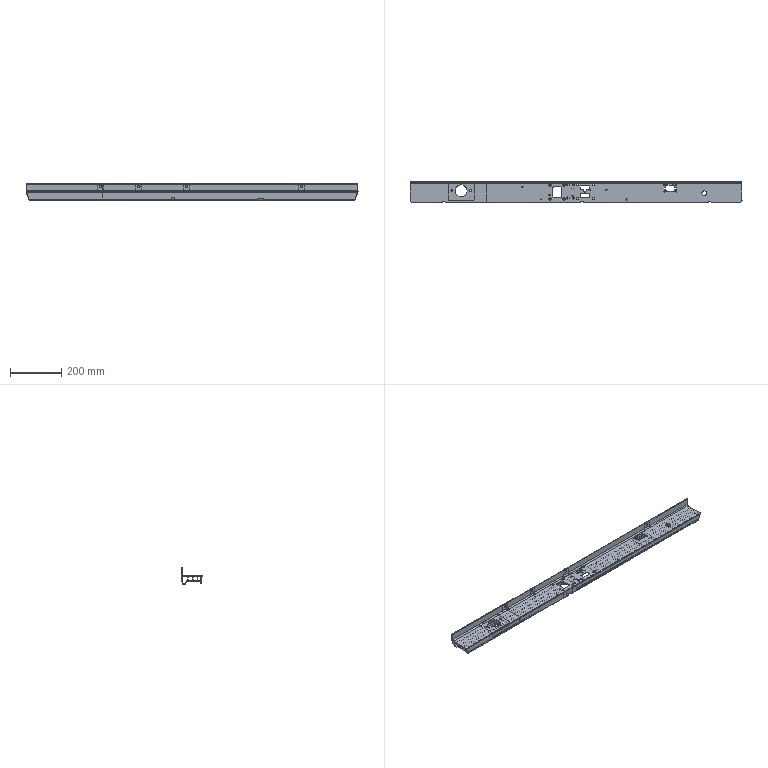NC program | NX | posted with a generic post | part box 1301 x 81.1 x 63 mm
Lines 13798 to 14822 of 19815:
(FIXED_CONTOUR_COPY , TOOL : D6)
N27582 T06 M6
N27584 G54
N27586 G17 G0 G90 X222.672 Y-32.604 B0. C0. S9500 M3
N27588 G43 Z30. H6
N27590 Z3.6
N27592 G94 G1 Z-0.54 F1000.
N27594 G2 X222.372 Y-32.084 R0.6
N27596 G1 Y-31.745 Z-0.522 F2500.
N27598 Y-31.55 Z-0.514
N27600 Y-31.069 Z-0.503
N27602 Y-30.589 Z-0.501
N27604 Y-30.108 Z-0.509
N27606 Y-29.559 Z-0.53
N27608 X222.401 Y-29.379 Z-0.579
N27610 X222.462 Y-29.117 Z-0.676
N27612 X222.481 Y-29.051 Z-0.705
N27614 Y-29.628 Z-0.675
N27616 Y-30.108 Z-0.657
N27618 Y-30.589 Z-0.647
N27620 Y-31.069 Z-0.648
N27622 Y-31.55 Z-0.659
N27624 Y-32.03 Z-0.681
N27626 Y-32.555 Z-0.715
N27628 X222.538 Y-32.748 Z-0.807
N27630 X222.61 Y-32.979 Z-0.916
N27632 X222.62 Y-33.005 Z-0.929
N27634 Y-32.489 Z-0.893
N27636 Y-32.03 Z-0.864
N27638 Y-31.739 Z-0.85
N27640 Y-31.55 Z-0.843
N27642 Y-31.069 Z-0.832
N27644 Y-30.589 Z-0.833
N27646 Y-30.108 Z-0.843
N27648 Y-29.65 Z-0.862
N27650 Y-28.617 Z-0.918
N27652 X222.719 Y-28.379 Z-1.062
N27654 X222.778 Y-28.245 Z-1.143
N27656 Y-28.438 Z-1.137
N27658 Y-28.909 Z-1.116
N27660 Y-29.628 Z-1.075
N27662 Y-30.108 Z-1.054
N27664 Y-30.589 Z-1.042
N27666 Y-31.069
N27668 Y-31.675 Z-1.058
N27670 Y-32.03 Z-1.075
N27672 Y-32.334 Z-1.094
N27674 Y-32.511 Z-1.103
N27676 Y-32.815 Z-1.125
N27678 Y-32.992 Z-1.132
N27680 Y-33.381 Z-1.153
N27682 X222.818 Y-33.463 Z-1.209
N27684 X222.95 Y-33.7 Z-1.384
N27686 Y-33.24 Z-1.368
N27688 Y-32.992 Z-1.355
N27690 Y-32.646 Z-1.341
N27692 Y-32.511 Z-1.331
N27694 Y-32.165 Z-1.314
N27696 Y-32.03 Z-1.305
N27698 Y-31.55 Z-1.283
N27700 Y-31.069 Z-1.271
N27702 Y-30.589 Z-1.272
N27704 Y-30.108 Z-1.284
N27706 Y-29.493 Z-1.314
N27708 Y-29.013 Z-1.341
N27710 Y-28.566 Z-1.361
N27712 Y-28.139 Z-1.369
N27714 Y-27.914 Z-1.372
N27716 X223.09 Y-27.662 Z-1.556
N27718 X223.127 Y-27.6 Z-1.603
N27720 Y-28.403 Z-1.594
N27722 Y-28.706 Z-1.589
N27724 Y-29.186 Z-1.569
N27726 Y-29.628 Z-1.543
N27728 Y-30.108 Z-1.52
N27730 Y-30.589 Z-1.506
N27732 Y-31.069
N27734 Y-31.55 Z-1.519
N27736 Y-32.511 Z-1.564
N27738 Y-32.992 Z-1.582
N27740 Y-33.472 Z-1.596
N27742 Y-33.953 Z-1.614
N27744 Y-34.011 Z-1.615
N27746 X223.153 Y-34.055 Z-1.649
N27748 X223.307 Y-34.181 Z-1.838
N27750 Y-33.738 Z-1.833
N27752 Y-33.207 Z-1.814
N27754 Y-32.776 Z-1.807
N27756 Y-32.511 Z-1.797
N27758 Y-32.295 Z-1.792
N27760 Y-32.03 Z-1.779
N27762 Y-31.55 Z-1.759
N27764 Y-31.069 Z-1.746
N27766 Y-30.589
N27768 Y-30.108 Z-1.76
N27770 Y-29.628 Z-1.783
N27772 Y-29.363 Z-1.798
N27774 Y-29.147 Z-1.804
N27776 Y-28.883 Z-1.815
N27778 Y-28.402 Z-1.823
N27780 Y-27.922 Z-1.828
N27782 Y-27.453 Z-1.826
N27784 Y-27.422 Z-1.827
N27786 X223.487 Y-27.271 Z-2.05
N27788 Y-28.099 Z-2.054
N27790 Y-28.614 Z-2.049
N27792 Y-29.06 Z-2.042
N27794 Y-29.54 Z-2.027
N27796 Y-30.108 Z-1.999
N27798 Y-30.589 Z-1.985
N27800 Y-31.069
N27802 Y-31.55 Z-1.999
N27804 Y-32.118 Z-2.022
N27806 Y-32.511 Z-2.03
N27808 Y-32.599 Z-2.034
N27810 Y-32.992 Z-2.041
N27812 Y-33.384 Z-2.045
N27814 Y-33.56 Z-2.052
N27816 Y-33.953 Z-2.054
N27818 Y-34.329 Z-2.059
N27820 X223.667 Y-34.478 Z-2.281
N27822 Y-33.863 Z-2.274
N27824 Y-33.383 Z-2.272
N27826 Y-32.992 Z-2.268
N27828 Y-32.6 Z-2.26
N27830 Y-32.511
N27832 Y-32.03 Z-2.252
N27834 Y-31.941
N27836 Y-31.55 Z-2.237
N27838 Y-31.069 Z-2.225
N27840 Y-30.589
N27842 Y-30.108 Z-2.238
N27844 Y-29.717 Z-2.257
N27846 Y-29.539 Z-2.258
N27848 Y-29.147 Z-2.268
N27850 Y-29.058
N27852 Y-28.667 Z-2.275
N27854 Y-28.276 Z-2.278
N27856 Y-27.617 Z-2.276
N27858 Y-27.121 Z-2.272
N27860 X223.848 Y-26.971 Z-2.494
N27862 Y-27.439 Z-2.498
N27864 Y-28.453 Z-2.499
N27866 Y-28.881 Z-2.494
N27868 Y-29.147
N27870 Y-29.361 Z-2.489
N27872 Y-29.895 Z-2.486
N27874 Y-30.108 Z-2.476
N27876 Y-30.589 Z-2.464
N27878 Y-31.069
N27880 Y-31.283 Z-2.471
N27882 Y-31.55 Z-2.474
N27884 Y-31.764 Z-2.482
N27886 Y-32.297 Z-2.483
N27888 Y-32.511 Z-2.488
N27890 Y-32.778
N27892 Y-33.205 Z-2.494
N27894 Y-33.953 Z-2.495
N27896 Y-34.626 Z-2.501
N27898 X224.029 Y-34.774 Z-2.722
N27900 Y-33.953 Z-2.717
N27902 Y-32.474 Z-2.714
N27904 Y-32.03 Z-2.712
N27906 Y-31.587
N27908 Y-31.069 Z-2.704
N27910 Y-30.552 Z-2.705
N27912 Y-30.072 Z-2.716
N27914 Y-29.628 Z-2.719
N27916 Y-28.63 Z-2.721
N27918 Y-27.225 Z-2.718
N27920 Y-26.821 Z-2.716
N27922 X224.211 Y-26.67 Z-2.941
N27924 Y-26.745 Z-2.937
N27926 Y-27.049 Z-2.942
N27928 Y-29.628 Z-2.946
N27930 Y-29.823 Z-2.944
N27932 Y-30.108 Z-2.946
N27934 Y-30.394 Z-2.945
N27936 Y-30.589 Z-2.941
N27938 Y-31.069 Z-2.942
N27940 Y-31.265 Z-2.945
N27942 Y-32.03 Z-2.94
N27944 Y-33.953 Z-2.941
N27946 Y-34.923 Z-2.943
N27948 X224.353 Y-35.038 Z-3.113
N27950 X224.4 Y-35.041 Z-3.168
N27952 Y-34.993 Z-3.165
N27954 Y-34.609 Z-3.167
N27956 Y-32.03 Z-3.169
N27958 Y-31.069 Z-3.175
N27960 Y-30.589 Z-3.173
N27962 Y-30.108 Z-3.175
N27964 Y-28.667 Z-3.169
N27966 Y-27.049 Z-3.168
N27968 Y-26.745 Z-3.162
N27970 Y-26.669 Z-3.166
N27972 Y-26.542
N27974 X224.555 Z-3.347
N27976 X224.598 Y-26.541 Z-3.39
N27978 Y-26.58 Z-3.388
N27980 Y-29.231 Z-3.391
N27982 Y-30.108 Z-3.395
N27984 Y-31.55
N27986 Y-32.511 Z-3.389
N27988 Y-35.054 Z-3.39
N27990 X224.81 Y-35.066 Z-3.602
N27992 Y-34.92 Z-3.597
N27994 Y-32.511
N27996 Y-31.55 Z-3.604
N27998 Y-31.089 Z-3.597
N28000 Y-30.57
N28002 Y-30.108 Z-3.604
N28004 Y-28.648 Z-3.597
N28006 Y-26.736
N28008 Y-26.53 Z-3.602
N28010 X225.034 Y-26.519 Z-3.791
N28012 Y-27.706 Z-3.792
N28014 Y-28.667
N28016 Y-29.628 Z-3.797
N28018 Y-31.848 Z-3.798
N28020 Y-32.49 Z-3.792
N28022 Y-34.433 Z-3.79
N28024 Y-35.074 Z-3.786
N28026 X225.136 Y-35.077 Z-3.858
N28028 X225.272 Y-35.082 Z-3.944
N28030 Y-34.4 Z-3.95
N28032 Y-32.958 Z-3.953
N28034 Y-32.511 Z-3.959
N28036 Y-31.977 Z-3.973
N28038 Y-31.82 Z-3.977
N28040 Y-31.55 Z-3.979
N28042 Y-30.075
N28044 Y-29.628 Z-3.967
N28046 Y-29.181 Z-3.959
N28048 Y-27.225 Z-3.95
N28050 Y-26.745 Z-3.953
N28052 Y-26.513 Z-3.957
N28054 X225.408 Y-26.511 Z-4.04
N28056 X225.523 Y-26.51 Z-4.107
N28058 Y-26.745 Z-4.104
N28060 Y-27.225 Z-4.102
N28062 Y-28.667 Z-4.108
N28064 Y-29.169 Z-4.112
N28066 Y-29.649 Z-4.124
N28068 Y-30.108 Z-4.143
N28070 Y-31.55
N28072 Y-31.84 Z-4.136
N28074 Y-32.028 Z-4.123
N28076 Y-32.511 Z-4.109
N28078 Y-32.992 Z-4.104
N28080 Y-34.433 Z-4.102
N28082 Y-35.087 Z-4.097
N28084 X225.781 Y-35.091 Z-4.25
N28086 Y-34.914 Z-4.247
N28088 Y-34.433 Z-4.249
N28090 Y-32.511 Z-4.251
N28092 Y-32.03 Z-4.264
N28094 Y-31.55 Z-4.293
N28096 Y-30.108
N28098 Y-29.628 Z-4.265
N28100 Y-29.147 Z-4.253
N28102 Y-26.743 Z-4.249
N28104 Y-26.507 Z-4.253
N28106 X226.047 Y-26.506 Z-4.386
N28108 Y-29.147
N28110 Y-29.651 Z-4.398
N28112 Y-30.108 Z-4.429
N28114 Y-31.55
N28116 Y-32.03 Z-4.395
N28118 Y-32.511 Z-4.387
N28120 Y-35.093 Z-4.386
N28122 X226.268 Y-35.095 Z-4.484
N28124 X226.322 Z-4.505
N28126 Y-34.954 Z-4.503
N28128 Y-32.405 Z-4.505
N28130 Y-32.03 Z-4.511
N28132 Y-31.55 Z-4.544
N28134 Y-31.444 Z-4.546
N28136 Y-30.108
N28138 Y-29.921 Z-4.528
N28140 Y-29.734 Z-4.52
N28142 Y-29.628 Z-4.514
N28144 Y-29.147 Z-4.504
N28146 Y-26.638
N28148 Y-26.504 Z-4.505
N28150 X226.512 Y-26.503 Z-4.58
N28152 X226.603 Z-4.609
N28154 Y-29.147 Z-4.608
N28156 Y-29.628 Z-4.616
N28158 Y-29.717 Z-4.619
N28160 Y-29.806 Z-4.627
N28162 Y-30.108 Z-4.646
N28164 Y-30.589 Z-4.649
N28166 Y-31.069
N28168 Y-31.55 Z-4.64
N28170 Y-32.03 Z-4.613
N28172 Y-32.511 Z-4.608
N28174 Y-34.948 Z-4.607
N28176 Y-35.097 Z-4.609
N28178 X226.89 Y-35.098 Z-4.694
N28180 Y-32.511
N28182 Y-32.03 Z-4.699
N28184 Y-31.769 Z-4.709
N28186 Y-31.55 Z-4.721
N28188 Y-31.288 Z-4.731
N28190 Y-31.069 Z-4.735
N28192 Y-30.37 Z-4.734
N28194 Y-30.108 Z-4.727
N28196 Y-29.999 Z-4.717
N28198 Y-29.628 Z-4.702
N28200 Y-29.147 Z-4.695
N28202 Y-26.502 Z-4.694
N28204 X227.001 Z-4.727
N28206 X227.182 Y-26.501 Z-4.761
N28208 Y-27.048 Z-4.76
N28210 Y-27.706 Z-4.762
N28212 Y-29.147 Z-4.763
N28214 Y-29.628 Z-4.771
N28216 Y-29.805 Z-4.777
N28218 Y-30.108 Z-4.792
N28220 Y-30.589 Z-4.8
N28222 Y-31.069
N28224 Y-31.423 Z-4.791
N28226 Y-32.03 Z-4.768
N28228 Y-32.511 Z-4.764
N28230 Y-34.914 Z-4.761
N28232 Y-35.099 Z-4.765
N28234 X227.476 Z-4.821
N28236 Y-34.448 Z-4.817
N28238 Y-32.496 Z-4.823
N28240 Y-32.001 Z-4.828
N28242 Y-31.55 Z-4.843
N28244 Y-31.069 Z-4.852
N28246 Y-30.559
N28248 Y-30.094 Z-4.847
N28250 Y-29.628 Z-4.831
N28252 Y-29.147 Z-4.822
N28254 Y-28.667 Z-4.817
N28256 Y-27.225 Z-4.818
N28258 Y-26.501 Z-4.813
N28260 X227.772 Y-26.5 Z-4.857
N28262 Y-26.732 Z-4.86
N28264 Y-27.225 Z-4.863
N28266 Y-28.739
N28268 Y-29.7 Z-4.873
N28270 Y-30.108 Z-4.883
N28272 Y-31.141 Z-4.884
N28274 Y-31.622 Z-4.878
N28276 Y-32.03 Z-4.869
N28278 Y-32.583 Z-4.865
N28280 Y-34.505 Z-4.862
N28282 Y-35.072 Z-4.866
N28284 Y-35.099 Z-4.863
N28286 X227.846 Y-35.1 Z-4.874
N28288 X227.98 Z-4.888
N28290 X228.07 Z-4.891
N28292 Y-33.953 Z-4.889
N28294 Y-32.03 Z-4.89
N28296 Y-31.069 Z-4.897
N28298 Y-30.108
N28300 Y-29.54 Z-4.893
N28302 Y-28.667 Z-4.889
N28304 Y-26.677 Z-4.888
N28306 Y-26.5 Z-4.891
N28308 X228.268 Z-4.897
N28310 X228.37 Z-4.899
N28312 Y-26.843 Z-4.897
N28314 Y-29.628 Z-4.898
N28316 Y-29.824 Z-4.9
N28318 Y-31.354
N28320 Y-32.03 Z-4.898
N28322 Y-35.1
N28324 X228.47 Z-4.9
N28326 X228.67
N28328 Y-26.5
N28330 X228.97
N28332 Y-35.1
N28334 X229.27
N28336 Y-26.5
N28338 X229.57
N28340 Y-35.1
N28342 X229.87
N28344 Y-26.5
N28346 X230.17
N28348 Y-35.1
N28350 X230.47
N28352 Y-26.5
N28354 X230.77
N28356 Y-35.1
N28358 X231.07
N28360 Y-26.5
N28362 X231.37
N28364 Y-35.1
N28366 X231.67
N28368 Y-26.5
N28370 X231.97
N28372 Y-35.1
N28374 X232.27
N28376 Y-26.5
N28378 X232.57
N28380 Y-35.1
N28382 X232.87
N28384 Y-26.5
N28386 X233.17
N28388 Y-35.1
N28390 X233.47
N28392 Y-26.5
N28394 X233.77
N28396 Y-35.1
N28398 X234.07
N28400 Y-26.5
N28402 X234.37
N28404 Y-35.1
N28406 X234.67
N28408 Y-26.5
N28410 X234.97
N28412 Y-35.1
N28414 X235.27
N28416 Y-26.5
N28418 X235.57
N28420 Y-35.1
N28422 X235.87
N28424 Y-26.5
N28426 X236.17
N28428 Y-35.1
N28430 X236.47
N28432 Y-26.5
N28434 X236.77
N28436 Y-35.1
N28438 X237.07
N28440 Y-26.5
N28442 X237.37
N28444 Y-35.1
N28446 X237.67
N28448 Y-26.5
N28450 X237.97
N28452 Y-35.1
N28454 X238.27
N28456 Y-26.5
N28458 X238.57
N28460 Y-35.1
N28462 X238.87 Z-4.899
N28464 Y-34.678 Z-4.9
N28466 Y-34.433 Z-4.897
N28468 Y-32.03 Z-4.898
N28470 Y-31.786 Z-4.9
N28472 Y-30.353
N28474 Y-30.108 Z-4.898
N28476 Y-26.5 Z-4.897
N28478 X239.17 Z-4.89
N28480 Y-27.642 Z-4.888
N28482 Y-29.628 Z-4.89
N28484 Y-30.589 Z-4.897
N28486 Y-31.55
N28488 Y-32.094 Z-4.892
N28490 Y-32.992 Z-4.888
N28492 Y-34.433
N28494 Y-34.561 Z-4.89
N28496 Y-34.931 Z-4.889
N28498 Y-35.101 Z-4.891
N28500 X239.23 Z-4.885
N28502 X239.236 Y-34.914
N28504 X239.237 Y-34.9
N28506 X239.308 Y-34.895 Z-4.876
N28508 X239.33 Y-34.887 Z-4.874
N28510 X239.336 Y-34.877 Z-4.873
N28512 X239.372 Y-34.844 Z-4.869
N28514 Y-35.1
N28516 X239.468 Z-4.854
N28518 Y-34.433 Z-4.86
N28520 Y-32.992
N28522 Y-32.008 Z-4.869
N28524 Y-31.55 Z-4.881
N28526 Y-30.589 Z-4.883
N28528 Y-30.086 Z-4.878
N28530 Y-29.606 Z-4.867
N28532 Y-29.147 Z-4.863
N28534 Y-27.225 Z-4.859
N28536 Y-26.723 Z-4.861
N28538 Y-26.5 Z-4.859
N28540 X239.724 Y-26.501 Z-4.824
N28542 X239.764 Z-4.817
N28544 Y-26.745 Z-4.813
N28546 Y-27.186 Z-4.812
N28548 Y-28.706 Z-4.815
N28550 Y-29.628 Z-4.824
N28552 Y-30.108 Z-4.84
N28554 Y-30.589 Z-4.848
N28556 Y-31.109 Z-4.846
N28558 Y-31.55 Z-4.84
N28560 Y-32.03 Z-4.824
N28562 Y-32.511 Z-4.816
N28564 Y-32.992 Z-4.813
N28566 Y-34.433
N28568 Y-34.947 Z-4.809
N28570 Y-35.099
N28572 X240.059 Y-35.098 Z-4.756
N28574 Y-34.585
N28576 Y-34.433 Z-4.757
N28578 Y-32.511 Z-4.758
N28580 Y-32.03 Z-4.765
N28582 Y-31.55 Z-4.783
N28584 Y-31.398 Z-4.785
N28586 Y-31.069 Z-4.796
N28588 Y-30.589
N28590 Y-30.284 Z-4.79
N28592 Y-29.628 Z-4.764
N28594 Y-28.995 Z-4.758
N28596 Y-26.745 Z-4.757
N28598 Y-26.501 Z-4.759
N28600 X240.214 Y-26.502 Z-4.727
N28602 X240.35 Z-4.687
N28604 Y-29.147
N28606 Y-29.628 Z-4.693
N28608 Y-29.841 Z-4.702
N28610 Y-30.108 Z-4.718
N28612 Y-30.322 Z-4.725
N28614 Y-30.589 Z-4.728
N28616 Y-31.069
N28618 Y-31.337 Z-4.724
N28620 Y-31.55 Z-4.716
N28622 Y-31.817 Z-4.701
N28624 Y-32.03 Z-4.693
N28626 Y-32.645 Z-4.688
N28628 Y-35.028 Z-4.687
N28630 Y-35.098 Z-4.688
N28632 X240.637 Y-35.096 Z-4.6
N28634 Y-32.446 Z-4.601
N28636 Y-32.03 Z-4.606
N28638 Y-31.55 Z-4.634
N28640 Y-31.069 Z-4.642
N28642 Y-30.459 Z-4.641
N28644 Y-30.108 Z-4.637
N28646 Y-29.628 Z-4.608
N28648 Y-29.147 Z-4.601
N28650 Y-26.503
N28652 X240.703 Z-4.58
N28654 X240.916 Y-26.504 Z-4.496
N28656 Y-26.714 Z-4.494
N28658 Y-29.209 Z-4.495
N28660 Y-29.628 Z-4.505
N28662 Y-29.899 Z-4.517
N28664 Y-30.108 Z-4.537
N28666 Y-31.069
N28668 Y-31.55 Z-4.535
N28670 Y-31.76 Z-4.513
N28672 Y-32.03 Z-4.502
N28674 Y-32.511 Z-4.494
N28676 Y-34.937
N28678 Y-35.095 Z-4.496
N28680 X241.039 Y-35.094 Z-4.444
N28682 X241.191 Y-35.093 Z-4.375
N28684 Y-32.511 Z-4.376
N28686 Y-32.029 Z-4.384
N28688 Y-31.55 Z-4.418
N28690 Y-30.108 Z-4.42
N28692 Y-29.628 Z-4.388
N28694 Y-29.145 Z-4.378
N28696 Y-26.505 Z-4.376
N28698 X241.456 Y-26.507 Z-4.238
N28700 Y-26.782 Z-4.236
N28702 Y-27.225 Z-4.238
N28704 Y-28.704
N28706 Y-29.147 Z-4.241
N28708 Y-29.628 Z-4.257
N28710 Y-30.108 Z-4.281
N28712 Y-31.55
N28714 Y-32.03 Z-4.25
N28716 Y-32.511 Z-4.241
N28718 Y-32.992 Z-4.239
N28720 Y-33.915
N28722 Y-34.914 Z-4.236
N28724 Y-35.09 Z-4.24
N28726 X241.683 Y-35.088 Z-4.11
N28728 X241.714 Y-35.087 Z-4.092
N28730 Y-34.433 Z-4.087
N28732 Y-32.511 Z-4.097
N28734 Y-31.966 Z-4.109
N28736 Y-31.55 Z-4.129
N28738 Y-30.108
N28740 Y-29.781 Z-4.123
N28742 Y-29.628 Z-4.114
N28744 Y-29.147 Z-4.098
N28746 Y-28.667 Z-4.092
N28748 Y-27.225 Z-4.091
N28750 Y-26.509 Z-4.085
N28752 X241.964 Y-26.513 Z-3.937
N28754 Y-26.553
N28756 Y-26.561 Z-3.935
N28758 Y-27.225 Z-3.94
N28760 Y-28.741 Z-3.941
N28762 Y-29.147 Z-3.946
N28764 Y-29.554 Z-3.958
N28766 Y-29.832 Z-3.962
N28768 Y-31.624
N28770 Y-32.03 Z-3.95
N28772 Y-32.511 Z-3.942
N28774 Y-34.433 Z-3.932
N28776 Y-34.914 Z-3.935
N28778 Y-35.083 Z-3.939
N28780 X242.138 Y-35.078 Z-3.818
N28782 X242.201 Y-35.074 Z-3.769
N28784 Y-34.374 Z-3.766
N28786 Y-32.511 Z-3.775
N28788 Y-31.55 Z-3.78
N28790 Y-30.529
N28792 Y-29.762
N28794 Y-29.147 Z-3.774
N28796 Y-27.706 Z-3.773
N28798 Y-26.523 Z-3.774
N28800 X242.425 Y-26.537 Z-3.584
N28802 Y-26.736 Z-3.579
N28804 Y-29.147 Z-3.58
N28806 Y-30.108 Z-3.586
N28808 Y-30.571 Z-3.579
N28810 Y-31.087
N28812 Y-31.55 Z-3.586
N28814 Y-32.511 Z-3.58
N28816 Y-34.931
N28818 Y-35.058 Z-3.584
N28820 X242.486 Y-35.052 Z-3.525
N28822 X242.637 Y-35.036 Z-3.372
N28824 Y-32.466
N28826 Y-31.505 Z-3.375
N28828 Y-30.108 Z-3.376
N28830 Y-28.622 Z-3.371
N28832 Y-26.573 Z-3.372
N28834 Y-26.543 Z-3.374
N28836 X242.66 Y-26.541 Z-3.351
N28838 X242.79 Y-26.526 Z-3.205
N28840 X242.834 Y-26.52 Z-3.152
N28842 Y-26.614
N28844 Y-26.693 Z-3.148
N28846 Y-28.186 Z-3.147
N28848 Y-29.628 Z-3.148
N28850 Y-30.108 Z-3.151
N28852 Y-30.728 Z-3.149
N28854 Y-31.55 Z-3.153
N28856 Y-32.852 Z-3.149
N28858 Y-34.947 Z-3.148
N28860 Y-35.098 Z-3.158
N28862 X242.852 Y-35.112 Z-3.139
N28864 X242.903 Y-35.158 Z-3.073
N28866 X243.022 Y-35.036 Z-2.92
N28868 Y-34.913 Z-2.917
N28870 Y-31.55 Z-2.921
N28872 Y-30.819 Z-2.916
N28874 Y-30.589 Z-2.915
N28876 Y-30.108 Z-2.92
N28878 Y-29.628 Z-2.918
N28880 Y-28.917 Z-2.919
N28882 Y-27.225 Z-2.92
N28884 Y-26.651 Z-2.922
N28886 X243.206 Y-26.813 Z-2.698
N28888 Y-27.706 Z-2.693
N28890 Y-28.667 Z-2.692
N28892 Y-29.202 Z-2.69
N28894 Y-29.628 Z-2.686
N28896 Y-30.053 Z-2.687
N28898 Y-30.589 Z-2.678
N28900 Y-31.069 Z-2.68
N28902 Y-31.605 Z-2.687
N28904 Y-32.03 Z-2.689
N28906 Y-34.848 Z-2.685
N28908 X243.386 Y-34.664 Z-2.456
N28910 Y-32.743 Z-2.46
N28912 Y-32.279 Z-2.456
N28914 Y-31.782 Z-2.455
N28916 Y-31.55 Z-2.45
N28918 Y-31.302 Z-2.447
N28920 Y-31.069 Z-2.44
N28922 Y-30.589 Z-2.438
N28924 Y-30.357 Z-2.444
N28926 Y-30.108 Z-2.447
N28928 Y-29.876 Z-2.456
N28930 Y-29.38 Z-2.458
N28932 Y-29.147 Z-2.463
N28934 Y-28.899
N28936 Y-28.435 Z-2.47
N28938 Y-27.458 Z-2.472
N28940 Y-27.225 Z-2.476
N28942 Y-26.972 Z-2.477
N28944 X243.567 Y-27.132 Z-2.257
N28946 Y-27.777 Z-2.249
N28948 Y-28.257 Z-2.248
N28950 Y-28.667 Z-2.243
N28952 Y-29.147 Z-2.235
N28954 Y-29.628 Z-2.226
N28956 Y-29.699
N28958 Y-30.108 Z-2.21
N28960 Y-30.589 Z-2.199
N28962 Y-31.069 Z-2.201
N28964 Y-31.479 Z-2.213
N28966 Y-32.03 Z-2.224
N28968 Y-32.921 Z-2.232
N28970 Y-33.953 Z-2.231
N28972 Y-34.48 Z-2.228
N28974 X243.747 Y-34.297 Z-2.
N28976 Y-33.472 Z-2.003
N28978 Y-33.366 Z-2.001
N28980 Y-32.992 Z-2.002
N28982 Y-32.137 Z-1.993
N28984 Y-31.656 Z-1.98
N28986 Y-31.069 Z-1.961
N28988 Y-30.589 Z-1.959
N28990 Y-30.108 Z-1.971
N28992 Y-29.522 Z-1.995
N28994 Y-29.147 Z-2.004
N28996 Y-29.041 Z-2.008
N28998 Y-28.667 Z-2.015
N29000 Y-28.293 Z-2.019
N29002 Y-28.08 Z-2.027
N29004 Y-27.693 Z-2.029
N29006 Y-27.291 Z-2.035
N29008 X243.843 Y-27.376 Z-1.917
N29010 X243.927 Y-27.462 Z-1.813
N29012 Y-27.706 Z-1.808
N29014 Y-27.903 Z-1.807
N29016 Y-28.186 Z-1.796
N29018 Y-28.469 Z-1.788
N29020 Y-28.864 Z-1.782
N29022 Y-29.147 Z-1.77
N29024 Y-29.345 Z-1.765
N29026 Y-29.628 Z-1.751
N29028 Y-30.108 Z-1.731
N29030 Y-30.589 Z-1.72
N29032 Y-31.069 Z-1.721
N29034 Y-31.55 Z-1.736
N29036 Y-31.833 Z-1.748
N29038 Y-32.314 Z-1.761
N29040 Y-32.992 Z-1.77
N29042 Y-33.189
N29044 Y-33.472 Z-1.774
N29046 Y-34.113 Z-1.772
N29048 X244.107 Y-33.93 Z-1.544
N29050 Y-33.472 Z-1.545
N29052 Y-32.49 Z-1.53
N29054 Y-32.01 Z-1.516
N29056 Y-31.55 Z-1.497
N29058 Y-31.069 Z-1.482
N29060 Y-30.589 Z-1.48
N29062 Y-30.108 Z-1.491
N29064 Y-29.628 Z-1.512
N29066 Y-29.147 Z-1.536
N29068 Y-28.646 Z-1.556
N29070 Y-28.186 Z-1.569
N29072 Y-27.647 Z-1.59
N29074 X244.134 Y-27.675 Z-1.556
N29076 X244.287 Y-27.944 Z-1.354
N29078 Y-28.186 Z-1.344
N29080 Y-28.473 Z-1.336
N29082 Y-28.667 Z-1.323
N29084 Y-28.991 Z-1.309
N29086 Y-29.147 Z-1.298
N29088 Y-29.628 Z-1.272
N29090 Y-30.108 Z-1.252
N29092 Y-30.589 Z-1.241
N29094 Y-31.069 Z-1.243
N29096 Y-31.639 Z-1.26
N29098 Y-32.186 Z-1.283
N29100 Y-32.644 Z-1.297
N29102 Y-33.488 Z-1.31
N29104 Y-33.658
N29106 Y-33.697 Z-1.312
N29108 X244.395 Y-33.444 Z-1.168
N29110 X244.467 Y-33.269 Z-1.071
N29112 Y-32.794 Z-1.063
N29114 Y-32.363 Z-1.05
N29116 Y-31.55 Z-1.017
N29118 Y-31.069 Z-1.004
N29120 Y-30.589 Z-1.002
N29122 Y-30.108 Z-1.012
N29124 Y-29.628 Z-1.033
N29126 Y-29.147 Z-1.061
N29128 Y-28.815 Z-1.084
N29130 Y-28.667 Z-1.091
N29132 Y-28.275 Z-1.117
N29134 X244.522 Y-28.391 Z-1.038
N29136 X244.612 Y-28.636 Z-0.905
N29138 X244.646 Y-28.748 Z-0.853
N29140 Y-29.147 Z-0.823
N29142 Y-29.624 Z-0.794
N29144 Y-29.894 Z-0.781
N29146 Y-30.106 Z-0.774
N29148 Y-30.629 Z-0.764
N29150 Y-31.114 Z-0.766
N29152 Y-31.577 Z-0.777
N29154 Y-32.504 Z-0.816
N29156 Y-32.79 Z-0.825
N29158 X244.741 Y-32.483 Z-0.687
N29160 X244.818 Y-32.167 Z-0.568
N29162 X244.824 Y-32.133 Z-0.559
N29164 Y-31.542 Z-0.537
N29166 Y-31.062 Z-0.528
N29168 Y-30.589
N29170 Y-30.108 Z-0.538
N29172 Y-29.625 Z-0.559
N29174 Y-29.416 Z-0.571
N29176 G3 X244.524 Y-28.897 R0.6
N29178 G1 Z3.6
N29180 G0 Z30.
N29182 X571.107 Y-28.717
N29184 Z3.6
N29186 G1 Z2.257 F1000.
N29188 Y-32.708 Z-0.41
N29190 Y-32.31 Z-0.331 F2500.
N29192 Y-31.978 Z-0.274
N29194 Y-31.832 Z-0.255
N29196 Y-31.342 Z-0.2
N29198 Y-31.266 Z-0.197
N29200 Y-30.853 Z-0.172
N29202 Y-30.435 Z-0.175
N29204 Y-30.363 Z-0.177
N29206 Y-29.93 Z-0.204
N29208 Y-29.383 Z-0.264
N29210 Y-29.072 Z-0.311
N29212 X571.13 Y-28.644 Z-0.535
N29214 X571.135 Y-28.584 Z-0.574
N29216 Y-28.943 Z-0.514
N29218 Y-29.475 Z-0.435
N29220 Y-29.987 Z-0.38
N29222 Y-30.363 Z-0.357
N29224 Y-30.49 Z-0.352
N29226 Y-30.853 Z-0.35
N29228 Y-31.211 Z-0.372
N29230 Y-31.342 Z-0.377
N29232 Y-31.71 Z-0.419
N29234 Y-31.832 Z-0.431
N29236 Y-32.004 Z-0.453
N29238 Y-32.322 Z-0.508
N29240 Y-32.748 Z-0.593
N29242 Y-32.811 Z-0.603
N29244 Y-33.147 Z-0.678
N29246 X571.16 Y-33.455 Z-0.902
N29248 X571.17 Y-33.546 Z-0.98
N29250 Y-33.301 Z-0.923
N29252 Y-33.223 Z-0.91
N29254 Y-32.811 Z-0.818
N29256 Y-32.667 Z-0.795
N29258 Y-32.322 Z-0.726
N29260 Y-32.01 Z-0.674
N29262 Y-31.832 Z-0.651
N29264 Y-31.64 Z-0.632
N29266 Y-31.342 Z-0.598
N29268 Y-31.143 Z-0.59
N29270 Y-30.853 Z-0.572
N29272 Y-30.559 Z-0.574
N29274 Y-30.363 Z-0.581
N29276 Y-30.059 Z-0.6
N29278 Y-29.55 Z-0.654
N29280 Y-29.026 Z-0.731
N29282 Y-28.665 Z-0.79
N29284 Y-28.267 Z-0.86
N29286 Y-28.167 Z-0.876
N29288 X571.198 Y-27.914 Z-1.103
N29290 X571.21 Y-27.831 Z-1.193
N29292 Y-27.88 Z-1.186
N29294 Y-27.923 Z-1.182
N29296 Y-28.262 Z-1.127
N29298 Y-28.312 Z-1.12
N29300 Y-28.404 Z-1.104
N29302 Y-28.5 Z-1.089
N29304 Y-28.764 Z-1.044
N29306 Y-29.124 Z-0.986
N29308 Y-29.639 Z-0.91
N29310 Y-30.142 Z-0.858
N29312 Y-30.363 Z-0.844
N29314 Y-30.639 Z-0.834
N29316 Y-30.853 Z-0.833
N29318 Y-31.063 Z-0.845
N29320 Y-31.342 Z-0.856
N29322 Y-31.558 Z-0.881
N29324 Y-31.829 Z-0.908
N29326 Y-32.016 Z-0.932
N29328 Y-32.322 Z-0.982
N29330 Y-32.572 Z-1.032
N29332 Y-32.811 Z-1.071
N29334 Y-33.11 Z-1.137
N29336 Y-33.301 Z-1.168
N29338 Y-33.399 Z-1.192
N29340 Y-33.452 Z-1.2
N29342 Y-33.543 Z-1.221
N29344 Y-33.632 Z-1.236
N29346 Y-33.798 Z-1.278
N29348 Y-33.867 Z-1.294
N29350 X571.221 Y-33.937 Z-1.37
N29352 X571.249 Y-34.09 Z-1.559
N29354 X571.255 Y-34.116 Z-1.599
N29356 Y-34.043 Z-1.586
N29358 Y-33.945 Z-1.563
N29360 Y-33.855 Z-1.547
N29362 Y-33.823 Z-1.54
N29364 Y-33.791 Z-1.535
N29366 Y-33.698 Z-1.511
N29368 Y-33.51 Z-1.479
N29370 Y-33.457 Z-1.467
N29372 Y-33.358 Z-1.452
N29374 Y-33.301 Z-1.438
N29376 Y-32.986 Z-1.387
N29378 Y-32.811 Z-1.348
N29380 Y-32.468 Z-1.293
N29382 Y-32.322 Z-1.264
N29384 Y-32.023 Z-1.216
N29386 Y-31.83 Z-1.191
N29388 Y-31.468 Z-1.155
N29390 Y-31.342 Z-1.141
N29392 Y-30.976 Z-1.127
N29394 Y-30.853 Z-1.119
N29396 Y-30.728 Z-1.12
N29398 Y-30.363 Z-1.134
N29400 Y-30.234 Z-1.142
N29402 Y-29.736 Z-1.193
N29404 Y-29.232 Z-1.266
N29406 Y-28.569 Z-1.374
N29408 Y-28.404 Z-1.399
N29410 Y-28.35 Z-1.409
N29412 Y-27.951 Z-1.467
N29414 Y-27.769 Z-1.483
N29416 Y-27.55 Z-1.516
N29418 X571.29 Y-27.389 Z-1.741
N29420 X571.301 Y-27.346 Z-1.812
N29422 Y-27.584 Z-1.794
N29424 Y-27.658 Z-1.783
N29426 Y-27.98 Z-1.755
N29428 Y-28.404 Z-1.697
N29430 Y-28.662 Z-1.658
N29432 Y-29.383 Z-1.542
N29434 Y-29.873 Z-1.474
N29436 Y-30.327 Z-1.428
N29438 Y-30.853 Z-1.408
N29440 Y-31.342 Z-1.428
N29442 Y-31.832 Z-1.477
N29444 Y-32.042 Z-1.505
N29446 Y-32.322 Z-1.548
N29448 Y-32.363 Z-1.557
N29450 Y-32.811 Z-1.628
N29452 Y-32.86 Z-1.639
N29454 Y-33.587 Z-1.758
N29456 Y-33.765 Z-1.789
N29458 Y-33.791 Z-1.796
N29460 Y-33.975 Z-1.824
N29462 Y-34.228 Z-1.87
N29464 Y-34.295 Z-1.884
N29466 X571.327 Y-34.392 Z-2.037
N29468 X571.335 Y-34.417 Z-2.076
N29470 X571.347 Y-34.448 Z-2.136
N29472 Y-34.361 Z-2.129
N29474 Y-34.281 Z-2.116
N29476 Y-34.163 Z-2.114
N29478 Y-33.894 Z-2.068
N29480 Y-33.791 Z-2.054
N29482 Y-33.673 Z-2.044
N29484 Y-33.424 Z-2.002
N29486 Y-33.301 Z-1.983
N29488 Y-33.183 Z-1.97
N29490 Y-32.811 Z-1.91
N29492 Y-32.693 Z-1.896
N29494 Y-32.322 Z-1.837
N29496 Y-32.204 Z-1.823
N29498 Y-31.985 Z-1.79
N29500 Y-31.832 Z-1.77
N29502 Y-31.46 Z-1.733
N29504 Y-31.401 Z-1.722
N29506 Y-31.283 Z-1.72
N29508 Y-30.853 Z-1.703
N29510 Y-30.363 Z-1.721
N29512 Y-29.873 Z-1.772
N29514 Y-29.501 Z-1.825
N29516 Y-29.383 Z-1.838
N29518 Y-29.012 Z-1.898
N29520 Y-28.894 Z-1.912
N29522 Y-28.522 Z-1.969
N29524 Y-28.286 Z-1.989
N29526 Y-27.972 Z-2.031
N29528 Y-27.687 Z-2.056
N29530 Y-27.542 Z-2.066
N29532 Y-27.424 Z-2.071
N29534 Y-27.312
N29536 Y-27.182 Z-2.081
N29538 X571.391 Y-27.058 Z-2.319
N29540 X571.394 Y-27.051 Z-2.336
N29542 Y-27.084 Z-2.331
N29544 Y-27.133 Z-2.328
N29546 Y-27.424 Z-2.327
N29548 Y-27.734 Z-2.314
N29550 Y-27.942 Z-2.297
N29552 Y-28.094 Z-2.277
N29554 Y-28.404 Z-2.253
N29556 Y-28.714 Z-2.224
N29558 Y-28.894 Z-2.196
N29560 Y-29.203 Z-2.161
N29562 Y-29.383 Z-2.132
N29564 Y-29.693 Z-2.095
N29566 Y-29.873 Z-2.069
N29568 Y-30.053 Z-2.051
N29570 Y-30.363 Z-2.016
N29572 Y-30.518 Z-2.012
N29574 Y-30.853 Z-1.999
N29576 Y-31.187 Z-2.012
N29578 Y-31.497 Z-2.018
N29580 Y-31.652 Z-2.048
N29582 Y-31.832 Z-2.066
N29584 Y-32.012 Z-2.092
N29586 Y-32.322 Z-2.127
N29588 Y-32.502 Z-2.155
N29590 Y-32.811 Z-2.192
N29592 Y-32.991 Z-2.221
N29594 Y-33.301 Z-2.254
N29596 Y-33.481 Z-2.283
N29598 Y-33.791 Z-2.308
N29600 Y-33.971 Z-2.338
N29602 Y-34.126
N29604 Y-34.281 Z-2.341
N29606 Y-34.343 Z-2.352
N29608 Y-34.524 Z-2.363
N29610 Y-34.565 Z-2.369
N29612 X571.442 Y-34.654 Z-2.598
N29614 Y-34.617 Z-2.593
N29616 Y-34.325 Z-2.575
N29618 Y-34.281 Z-2.567
N29620 Y-34.03 Z-2.562
N29622 Y-33.779 Z-2.561
N29624 Y-33.289 Z-2.522